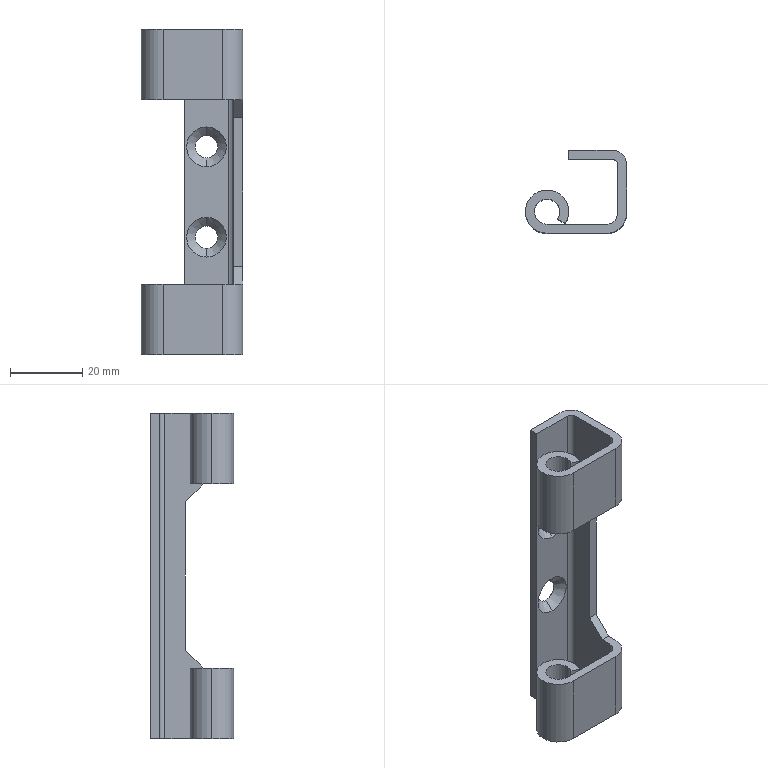Part | NX | features BREP 1 | 1 solid | 44 faces | box 28 x 23 x 90 mm | volume 10200 mm3 | cylinder 22 | plane 18 | cone 4 | commonest cylinder face diameters 7 x6 12 x6 6.2 x4 6 x2 11 x2 3 x1
STEP:
#1=CARTESIAN_POINT('',(6.,0.,-25.5));
#2=VERTEX_POINT('',#1);
#3=CARTESIAN_POINT('',(6.,0.,-45.));
#4=VERTEX_POINT('',#3);
#5=CARTESIAN_POINT('',(6.,0.,45.));
#6=DIRECTION('',(0.,0.,-1.));
#7=VECTOR('',#6,1000.);
#8=LINE('',#5,#7);
#9=EDGE_CURVE('',#2,#4,#8,.T.);
#10=ORIENTED_EDGE('',*,*,#9,.F.);
#11=CARTESIAN_POINT('',(5.029,-3.273,-25.5));
#12=VERTEX_POINT('',#11);
#13=CARTESIAN_POINT('',(0.0004653,0.,-25.5));
#14=DIRECTION('',(0.,0.,1.));
#15=DIRECTION('',(0.8381,-0.5456,0.));
#16=AXIS2_PLACEMENT_3D('',#13,#14,#15);
#17=CIRCLE('',#16,6.);
#18=EDGE_CURVE('',#12,#2,#17,.T.);
#19=ORIENTED_EDGE('',*,*,#18,.F.);
#20=CARTESIAN_POINT('',(5.029,-3.273,-45.));
#21=VERTEX_POINT('',#20);
#22=CARTESIAN_POINT('',(5.029,-3.273,-25.5));
#23=DIRECTION('',(0.,0.,-1.));
#24=VECTOR('',#23,1000.);
#25=LINE('',#22,#24);
#26=EDGE_CURVE('',#12,#21,#25,.T.);
#27=ORIENTED_EDGE('',*,*,#26,.T.);
#28=CARTESIAN_POINT('',(0.0004653,0.,-45.));
#29=DIRECTION('',(0.,0.,1.));
#30=DIRECTION('',(0.8381,-0.5456,0.));
#31=AXIS2_PLACEMENT_3D('',#28,#29,#30);
#32=CIRCLE('',#31,6.);
#33=EDGE_CURVE('',#21,#4,#32,.T.);
#34=ORIENTED_EDGE('',*,*,#33,.T.);
#35=EDGE_LOOP('',(#10,#19,#27,#34));
#36=FACE_BOUND('',#35,.T.);
#37=CARTESIAN_POINT('',(0.0004653,0.,45.));
#38=DIRECTION('',(0.,0.,-1.));
#39=DIRECTION('',(-1.,0.,0.));
#40=AXIS2_PLACEMENT_3D('',#37,#38,#39);
#41=CYLINDRICAL_SURFACE('',#40,6.);
#42=ADVANCED_FACE('',(#36),#41,.T.);
#43=CARTESIAN_POINT('',(16.5,-6.,-25.5));
#44=VERTEX_POINT('',#43);
#45=CARTESIAN_POINT('',(16.5,-6.,-45.));
#46=VERTEX_POINT('',#45);
#47=CARTESIAN_POINT('',(16.5,-6.,-25.5));
#48=DIRECTION('',(0.,0.,-1.));
#49=VECTOR('',#48,1000.);
#50=LINE('',#47,#49);
#51=EDGE_CURVE('',#44,#46,#50,.T.);
#52=ORIENTED_EDGE('',*,*,#51,.F.);
#53=CARTESIAN_POINT('',(0.0004653,-6.,-25.5));
#54=VERTEX_POINT('',#53);
#55=CARTESIAN_POINT('',(0.0004653,-6.,-25.5));
#56=DIRECTION('',(1.,0.,0.));
#57=VECTOR('',#56,1000.);
#58=LINE('',#55,#57);
#59=EDGE_CURVE('',#54,#44,#58,.T.);
#60=ORIENTED_EDGE('',*,*,#59,.F.);
#61=CARTESIAN_POINT('',(0.0004653,-6.,-45.));
#62=VERTEX_POINT('',#61);
#63=CARTESIAN_POINT('',(0.0004653,-6.,-25.5));
#64=DIRECTION('',(0.,0.,-1.));
#65=VECTOR('',#64,1000.);
#66=LINE('',#63,#65);
#67=EDGE_CURVE('',#54,#62,#66,.T.);
#68=ORIENTED_EDGE('',*,*,#67,.T.);
#69=CARTESIAN_POINT('',(0.0004653,-6.,-45.));
#70=DIRECTION('',(1.,0.,0.));
#71=VECTOR('',#70,1000.);
#72=LINE('',#69,#71);
#73=EDGE_CURVE('',#62,#46,#72,.T.);
#74=ORIENTED_EDGE('',*,*,#73,.T.);
#75=EDGE_LOOP('',(#52,#60,#68,#74));
#76=FACE_BOUND('',#75,.T.);
#77=CARTESIAN_POINT('',(0.0004653,-6.,45.));
#78=DIRECTION('',(0.,1.,0.));
#79=DIRECTION('',(0.,0.,1.));
#80=AXIS2_PLACEMENT_3D('',#77,#78,#79);
#81=PLANE('',#80);
#82=ADVANCED_FACE('',(#76),#81,.F.);
#83=CARTESIAN_POINT('',(16.5,-3.5,-25.5));
#84=VERTEX_POINT('',#83);
#85=CARTESIAN_POINT('',(0.0004653,-3.5,-25.5));
#86=VERTEX_POINT('',#85);
#87=CARTESIAN_POINT('',(16.5,-3.5,-25.5));
#88=DIRECTION('',(-1.,0.,0.));
#89=VECTOR('',#88,1000.);
#90=LINE('',#87,#89);
#91=EDGE_CURVE('',#84,#86,#90,.T.);
#92=ORIENTED_EDGE('',*,*,#91,.F.);
#93=CARTESIAN_POINT('',(16.5,-3.5,-45.));
#94=VERTEX_POINT('',#93);
#95=CARTESIAN_POINT('',(16.5,-3.5,-25.5));
#96=DIRECTION('',(0.,0.,-1.));
#97=VECTOR('',#96,1000.);
#98=LINE('',#95,#97);
#99=EDGE_CURVE('',#84,#94,#98,.T.);
#100=ORIENTED_EDGE('',*,*,#99,.T.);
#101=CARTESIAN_POINT('',(0.0004653,-3.5,-45.));
#102=VERTEX_POINT('',#101);
#103=CARTESIAN_POINT('',(16.5,-3.5,-45.));
#104=DIRECTION('',(-1.,0.,0.));
#105=VECTOR('',#104,1000.);
#106=LINE('',#103,#105);
#107=EDGE_CURVE('',#94,#102,#106,.T.);
#108=ORIENTED_EDGE('',*,*,#107,.T.);
#109=CARTESIAN_POINT('',(0.0004653,-3.5,-25.5));
#110=DIRECTION('',(0.,0.,-1.));
#111=VECTOR('',#110,1000.);
#112=LINE('',#109,#111);
#113=EDGE_CURVE('',#86,#102,#112,.T.);
#114=ORIENTED_EDGE('',*,*,#113,.F.);
#115=EDGE_LOOP('',(#92,#100,#108,#114));
#116=FACE_BOUND('',#115,.T.);
#117=CARTESIAN_POINT('',(16.5,-3.5,45.));
#118=DIRECTION('',(0.,-1.,0.));
#119=DIRECTION('',(0.,0.,-1.));
#120=AXIS2_PLACEMENT_3D('',#117,#118,#119);
#121=PLANE('',#120);
#122=ADVANCED_FACE('',(#116),#121,.F.);
#123=CARTESIAN_POINT('',(-3.5,0.000000072,-25.5));
#124=VERTEX_POINT('',#123);
#125=CARTESIAN_POINT('',(-3.5,0.000000072,-45.));
#126=VERTEX_POINT('',#125);
#127=CARTESIAN_POINT('',(-3.5,0.000000072,45.));
#128=DIRECTION('',(0.,0.,-1.));
#129=VECTOR('',#128,1000.);
#130=LINE('',#127,#129);
#131=EDGE_CURVE('',#124,#126,#130,.T.);
#132=ORIENTED_EDGE('',*,*,#131,.F.);
#133=CARTESIAN_POINT('',(0.0004654,0.000000072,-25.5));
#134=DIRECTION('',(0.,0.,1.));
#135=DIRECTION('',(0.8166,-0.5772,0.));
#136=AXIS2_PLACEMENT_3D('',#133,#134,#135);
#137=CIRCLE('',#136,3.5);
#138=EDGE_CURVE('',#124,#86,#137,.T.);
#139=ORIENTED_EDGE('',*,*,#138,.T.);
#140=ORIENTED_EDGE('',*,*,#113,.T.);
#141=CARTESIAN_POINT('',(0.0004654,0.000000072,-45.));
#142=DIRECTION('',(0.,0.,1.));
#143=DIRECTION('',(0.8166,-0.5772,0.));
#144=AXIS2_PLACEMENT_3D('',#141,#142,#143);
#145=CIRCLE('',#144,3.5);
#146=EDGE_CURVE('',#126,#102,#145,.T.);
#147=ORIENTED_EDGE('',*,*,#146,.F.);
#148=EDGE_LOOP('',(#132,#139,#140,#147));
#149=FACE_BOUND('',#148,.T.);
#150=CARTESIAN_POINT('',(0.0004654,0.000000072,45.));
#151=DIRECTION('',(0.,0.,-1.));
#152=DIRECTION('',(-1.,0.,0.));
#153=AXIS2_PLACEMENT_3D('',#150,#151,#152);
#154=CYLINDRICAL_SURFACE('',#153,3.5);
#155=ADVANCED_FACE('',(#149),#154,.F.);
#156=CARTESIAN_POINT('',(2.859,-2.02,-25.5));
#157=VERTEX_POINT('',#156);
#158=CARTESIAN_POINT('',(2.859,-2.02,-25.5));
#159=DIRECTION('',(0.866,-0.5,0.));
#160=VECTOR('',#159,1000.);
#161=LINE('',#158,#160);
#162=EDGE_CURVE('',#157,#12,#161,.T.);
#163=ORIENTED_EDGE('',*,*,#162,.F.);
#164=CARTESIAN_POINT('',(2.859,-2.02,-45.));
#165=VERTEX_POINT('',#164);
#166=CARTESIAN_POINT('',(2.859,-2.02,-25.5));
#167=DIRECTION('',(0.,0.,-1.));
#168=VECTOR('',#167,1000.);
#169=LINE('',#166,#168);
#170=EDGE_CURVE('',#157,#165,#169,.T.);
#171=ORIENTED_EDGE('',*,*,#170,.T.);
#172=CARTESIAN_POINT('',(2.859,-2.02,-45.));
#173=DIRECTION('',(0.866,-0.5,0.));
#174=VECTOR('',#173,1000.);
#175=LINE('',#172,#174);
#176=EDGE_CURVE('',#165,#21,#175,.T.);
#177=ORIENTED_EDGE('',*,*,#176,.T.);
#178=ORIENTED_EDGE('',*,*,#26,.F.);
#179=EDGE_LOOP('',(#163,#171,#177,#178));
#180=FACE_BOUND('',#179,.T.);
#181=CARTESIAN_POINT('',(2.859,-2.02,45.));
#182=DIRECTION('',(0.5,0.866,0.));
#183=DIRECTION('',(-0.866,0.5,0.));
#184=AXIS2_PLACEMENT_3D('',#181,#182,#183);
#185=PLANE('',#184);
#186=ADVANCED_FACE('',(#180),#185,.F.);
#187=CARTESIAN_POINT('',(12.,16.9,-9.4));
#188=VERTEX_POINT('',#187);
#189=CARTESIAN_POINT('',(12.,14.5,-7.));
#190=VERTEX_POINT('',#189);
#191=CARTESIAN_POINT('',(12.,16.9,-9.4));
#192=DIRECTION('',(0.,-0.7071,0.7071));
#193=VECTOR('',#192,1000.);
#194=LINE('',#191,#193);
#195=EDGE_CURVE('',#188,#190,#194,.T.);
#196=ORIENTED_EDGE('',*,*,#195,.F.);
#197=CARTESIAN_POINT('',(12.,16.9,-15.6));
#198=VERTEX_POINT('',#197);
#199=CARTESIAN_POINT('',(12.,16.9,-12.5));
#200=DIRECTION('',(0.,-1.,0.));
#201=DIRECTION('',(0.,0.,-1.));
#202=AXIS2_PLACEMENT_3D('',#199,#200,#201);
#203=CIRCLE('',#202,3.1);
#204=EDGE_CURVE('',#198,#188,#203,.T.);
#205=ORIENTED_EDGE('',*,*,#204,.F.);
#206=CARTESIAN_POINT('',(12.,14.5,-18.));
#207=VERTEX_POINT('',#206);
#208=CARTESIAN_POINT('',(12.,16.9,-15.6));
#209=DIRECTION('',(0.,-0.7071,-0.7071));
#210=VECTOR('',#209,1000.);
#211=LINE('',#208,#210);
#212=EDGE_CURVE('',#198,#207,#211,.T.);
#213=ORIENTED_EDGE('',*,*,#212,.T.);
#214=CARTESIAN_POINT('',(12.,14.5,-12.5));
#215=DIRECTION('',(0.,-1.,0.));
#216=DIRECTION('',(0.,0.,-1.));
#217=AXIS2_PLACEMENT_3D('',#214,#215,#216);
#218=CIRCLE('',#217,5.5);
#219=EDGE_CURVE('',#207,#190,#218,.T.);
#220=ORIENTED_EDGE('',*,*,#219,.T.);
#221=EDGE_LOOP('',(#196,#205,#213,#220));
#222=FACE_BOUND('',#221,.T.);
#223=CARTESIAN_POINT('',(12.,16.9,-12.5));
#224=DIRECTION('',(0.,-1.,0.));
#225=DIRECTION('',(0.,0.,-1.));
#226=AXIS2_PLACEMENT_3D('',#223,#224,#225);
#227=CONICAL_SURFACE('',#226,3.1,0.7854);
#228=ADVANCED_FACE('',(#222),#227,.F.);
#229=CARTESIAN_POINT('',(12.,16.9,15.6));
#230=VERTEX_POINT('',#229);
#231=CARTESIAN_POINT('',(12.,14.5,18.));
#232=VERTEX_POINT('',#231);
#233=CARTESIAN_POINT('',(12.,16.9,15.6));
#234=DIRECTION('',(0.,-0.7071,0.7071));
#235=VECTOR('',#234,1000.);
#236=LINE('',#233,#235);
#237=EDGE_CURVE('',#230,#232,#236,.T.);
#238=ORIENTED_EDGE('',*,*,#237,.F.);
#239=CARTESIAN_POINT('',(12.,16.9,9.4));
#240=VERTEX_POINT('',#239);
#241=CARTESIAN_POINT('',(12.,16.9,12.5));
#242=DIRECTION('',(0.,-1.,0.));
#243=DIRECTION('',(0.,0.,-1.));
#244=AXIS2_PLACEMENT_3D('',#241,#242,#243);
#245=CIRCLE('',#244,3.1);
#246=EDGE_CURVE('',#240,#230,#245,.T.);
#247=ORIENTED_EDGE('',*,*,#246,.F.);
#248=CARTESIAN_POINT('',(12.,14.5,7.));
#249=VERTEX_POINT('',#248);
#250=CARTESIAN_POINT('',(12.,16.9,9.4));
#251=DIRECTION('',(0.,-0.7071,-0.7071));
#252=VECTOR('',#251,1000.);
#253=LINE('',#250,#252);
#254=EDGE_CURVE('',#240,#249,#253,.T.);
#255=ORIENTED_EDGE('',*,*,#254,.T.);
#256=CARTESIAN_POINT('',(12.,14.5,12.5));
#257=DIRECTION('',(0.,-1.,0.));
#258=DIRECTION('',(0.,0.,-1.));
#259=AXIS2_PLACEMENT_3D('',#256,#257,#258);
#260=CIRCLE('',#259,5.5);
#261=EDGE_CURVE('',#249,#232,#260,.T.);
#262=ORIENTED_EDGE('',*,*,#261,.T.);
#263=EDGE_LOOP('',(#238,#247,#255,#262));
#264=FACE_BOUND('',#263,.T.);
#265=CARTESIAN_POINT('',(12.,16.9,12.5));
#266=DIRECTION('',(0.,-1.,0.));
#267=DIRECTION('',(0.,0.,-1.));
#268=AXIS2_PLACEMENT_3D('',#265,#266,#267);
#269=CONICAL_SURFACE('',#268,3.1,0.7854);
#270=ADVANCED_FACE('',(#264),#269,.F.);
#271=CARTESIAN_POINT('',(12.,17.,-9.4));
#272=VERTEX_POINT('',#271);
#273=CARTESIAN_POINT('',(12.,14.5,-9.4));
#274=DIRECTION('',(0.,-1.,0.));
#275=VECTOR('',#274,1000.);
#276=LINE('',#273,#275);
#277=EDGE_CURVE('',#272,#188,#276,.T.);
#278=ORIENTED_EDGE('',*,*,#277,.F.);
#279=CARTESIAN_POINT('',(12.,17.,-15.6));
#280=VERTEX_POINT('',#279);
#281=CARTESIAN_POINT('',(12.,17.,-12.5));
#282=DIRECTION('',(0.,1.,0.));
#283=DIRECTION('',(0.,0.,-1.));
#284=AXIS2_PLACEMENT_3D('',#281,#282,#283);
#285=CIRCLE('',#284,3.1);
#286=EDGE_CURVE('',#272,#280,#285,.T.);
#287=ORIENTED_EDGE('',*,*,#286,.T.);
#288=CARTESIAN_POINT('',(12.,14.5,-15.6));
#289=DIRECTION('',(0.,-1.,0.));
#290=VECTOR('',#289,1000.);
#291=LINE('',#288,#290);
#292=EDGE_CURVE('',#280,#198,#291,.T.);
#293=ORIENTED_EDGE('',*,*,#292,.T.);
#294=ORIENTED_EDGE('',*,*,#204,.T.);
#295=EDGE_LOOP('',(#278,#287,#293,#294));
#296=FACE_BOUND('',#295,.T.);
#297=CARTESIAN_POINT('',(12.,14.5,-12.5));
#298=DIRECTION('',(0.,-1.,0.));
#299=DIRECTION('',(0.,0.,-1.));
#300=AXIS2_PLACEMENT_3D('',#297,#298,#299);
#301=CYLINDRICAL_SURFACE('',#300,3.1);
#302=ADVANCED_FACE('',(#296),#301,.F.);
#303=CARTESIAN_POINT('',(12.,17.,15.6));
#304=VERTEX_POINT('',#303);
#305=CARTESIAN_POINT('',(12.,14.5,15.6));
#306=DIRECTION('',(0.,-1.,0.));
#307=VECTOR('',#306,1000.);
#308=LINE('',#305,#307);
#309=EDGE_CURVE('',#304,#230,#308,.T.);
#310=ORIENTED_EDGE('',*,*,#309,.F.);
#311=CARTESIAN_POINT('',(12.,17.,9.4));
#312=VERTEX_POINT('',#311);
#313=CARTESIAN_POINT('',(12.,17.,12.5));
#314=DIRECTION('',(0.,1.,0.));
#315=DIRECTION('',(0.,0.,-1.));
#316=AXIS2_PLACEMENT_3D('',#313,#314,#315);
#317=CIRCLE('',#316,3.1);
#318=EDGE_CURVE('',#304,#312,#317,.T.);
#319=ORIENTED_EDGE('',*,*,#318,.T.);
#320=CARTESIAN_POINT('',(12.,14.5,9.4));
#321=DIRECTION('',(0.,-1.,0.));
#322=VECTOR('',#321,1000.);
#323=LINE('',#320,#322);
#324=EDGE_CURVE('',#312,#240,#323,.T.);
#325=ORIENTED_EDGE('',*,*,#324,.T.);
#326=ORIENTED_EDGE('',*,*,#246,.T.);
#327=EDGE_LOOP('',(#310,#319,#325,#326));
#328=FACE_BOUND('',#327,.T.);
#329=CARTESIAN_POINT('',(12.,14.5,12.5));
#330=DIRECTION('',(0.,-1.,0.));
#331=DIRECTION('',(0.,0.,-1.));
#332=AXIS2_PLACEMENT_3D('',#329,#330,#331);
#333=CYLINDRICAL_SURFACE('',#332,3.1);
#334=ADVANCED_FACE('',(#328),#333,.F.);
#335=CARTESIAN_POINT('',(22.,-0.5,-25.5));
#336=VERTEX_POINT('',#335);
#337=CARTESIAN_POINT('',(16.5,-0.5,-25.5));
#338=DIRECTION('',(0.,0.,1.));
#339=DIRECTION('',(0.,-1.,0.));
#340=AXIS2_PLACEMENT_3D('',#337,#338,#339);
#341=CIRCLE('',#340,5.5);
#342=EDGE_CURVE('',#44,#336,#341,.T.);
#343=ORIENTED_EDGE('',*,*,#342,.F.);
#344=ORIENTED_EDGE('',*,*,#51,.T.);
#345=CARTESIAN_POINT('',(22.,-0.5,-45.));
#346=VERTEX_POINT('',#345);
#347=CARTESIAN_POINT('',(16.5,-0.5,-45.));
#348=DIRECTION('',(0.,0.,1.));
#349=DIRECTION('',(0.,-1.,0.));
#350=AXIS2_PLACEMENT_3D('',#347,#348,#349);
#351=CIRCLE('',#350,5.5);
#352=EDGE_CURVE('',#46,#346,#351,.T.);
#353=ORIENTED_EDGE('',*,*,#352,.T.);
#354=CARTESIAN_POINT('',(22.,-0.5,-25.5));
#355=DIRECTION('',(0.,0.,-1.));
#356=VECTOR('',#355,1000.);
#357=LINE('',#354,#356);
#358=EDGE_CURVE('',#336,#346,#357,.T.);
#359=ORIENTED_EDGE('',*,*,#358,.F.);
#360=EDGE_LOOP('',(#343,#344,#353,#359));
#361=FACE_BOUND('',#360,.T.);
#362=CARTESIAN_POINT('',(16.5,-0.5,45.));
#363=DIRECTION('',(0.,0.,-1.));
#364=DIRECTION('',(-1.,0.,0.));
#365=AXIS2_PLACEMENT_3D('',#362,#363,#364);
#366=CYLINDRICAL_SURFACE('',#365,5.5);
#367=ADVANCED_FACE('',(#361),#366,.T.);
#368=CARTESIAN_POINT('',(22.,7.3,-20.55));
#369=VERTEX_POINT('',#368);
#370=CARTESIAN_POINT('',(22.,7.3,20.55));
#371=VERTEX_POINT('',#370);
#372=CARTESIAN_POINT('',(22.,7.3,-20.55));
#373=DIRECTION('',(0.,0.,1.));
#374=VECTOR('',#373,1000.);
#375=LINE('',#372,#374);
#376=EDGE_CURVE('',#369,#371,#375,.T.);
#377=ORIENTED_EDGE('',*,*,#376,.T.);
#378=CARTESIAN_POINT('',(19.5,7.3,20.55));
#379=VERTEX_POINT('',#378);
#380=CARTESIAN_POINT('',(22.,7.3,20.55));
#381=DIRECTION('',(-1.,0.,0.));
#382=VECTOR('',#381,1000.);
#383=LINE('',#380,#382);
#384=EDGE_CURVE('',#371,#379,#383,.T.);
#385=ORIENTED_EDGE('',*,*,#384,.T.);
#386=CARTESIAN_POINT('',(19.5,7.3,-20.55));
#387=VERTEX_POINT('',#386);
#388=CARTESIAN_POINT('',(19.5,7.3,20.55));
#389=DIRECTION('',(0.,0.,-1.));
#390=VECTOR('',#389,1000.);
#391=LINE('',#388,#390);
#392=EDGE_CURVE('',#379,#387,#391,.T.);
#393=ORIENTED_EDGE('',*,*,#392,.T.);
#394=CARTESIAN_POINT('',(22.,7.3,-20.55));
#395=DIRECTION('',(-1.,0.,0.));
#396=VECTOR('',#395,1000.);
#397=LINE('',#394,#396);
#398=EDGE_CURVE('',#369,#387,#397,.T.);
#399=ORIENTED_EDGE('',*,*,#398,.F.);
#400=EDGE_LOOP('',(#377,#385,#393,#399));
#401=FACE_BOUND('',#400,.T.);
#402=CARTESIAN_POINT('',(60.,7.3,-20.55));
#403=DIRECTION('',(0.,-1.,0.));
#404=DIRECTION('',(0.,0.,-1.));
#405=AXIS2_PLACEMENT_3D('',#402,#403,#404);
#406=PLANE('',#405);
#407=ADVANCED_FACE('',(#401),#406,.T.);
#408=CARTESIAN_POINT('',(22.,2.35,-25.5));
#409=VERTEX_POINT('',#408);
#410=CARTESIAN_POINT('',(22.,2.35,-25.5));
#411=DIRECTION('',(0.,0.7071,0.7071));
#412=VECTOR('',#411,1000.);
#413=LINE('',#410,#412);
#414=EDGE_CURVE('',#409,#369,#413,.T.);
#415=ORIENTED_EDGE('',*,*,#414,.T.);
#416=ORIENTED_EDGE('',*,*,#398,.T.);
#417=CARTESIAN_POINT('',(19.5,2.35,-25.5));
#418=VERTEX_POINT('',#417);
#419=CARTESIAN_POINT('',(19.5,7.3,-20.55));
#420=DIRECTION('',(0.,-0.7071,-0.7071));
#421=VECTOR('',#420,1000.);
#422=LINE('',#419,#421);
#423=EDGE_CURVE('',#387,#418,#422,.T.);
#424=ORIENTED_EDGE('',*,*,#423,.T.);
#425=CARTESIAN_POINT('',(22.,2.35,-25.5));
#426=DIRECTION('',(-1.,0.,0.));
#427=VECTOR('',#426,1000.);
#428=LINE('',#425,#427);
#429=EDGE_CURVE('',#409,#418,#428,.T.);
#430=ORIENTED_EDGE('',*,*,#429,.F.);
#431=EDGE_LOOP('',(#415,#416,#424,#430));
#432=FACE_BOUND('',#431,.T.);
#433=CARTESIAN_POINT('',(60.,2.35,-25.5));
#434=DIRECTION('',(0.,-0.7071,0.7071));
#435=DIRECTION('',(0.,-0.7071,-0.7071));
#436=AXIS2_PLACEMENT_3D('',#433,#434,#435);
#437=PLANE('',#436);
#438=ADVANCED_FACE('',(#432),#437,.T.);
#439=ORIENTED_EDGE('',*,*,#59,.T.);
#440=ORIENTED_EDGE('',*,*,#342,.T.);
#441=CARTESIAN_POINT('',(22.,-0.5,-25.5));
#442=DIRECTION('',(0.,1.,0.));
#443=VECTOR('',#442,1000.);
#444=LINE('',#441,#443);
#445=EDGE_CURVE('',#336,#409,#444,.T.);
#446=ORIENTED_EDGE('',*,*,#445,.T.);
#447=ORIENTED_EDGE('',*,*,#429,.T.);
#448=CARTESIAN_POINT('',(19.5,-0.5,-25.5));
#449=VERTEX_POINT('',#448);
#450=CARTESIAN_POINT('',(19.5,2.35,-25.5));
#451=DIRECTION('',(0.,-1.,0.));
#452=VECTOR('',#451,1000.);
#453=LINE('',#450,#452);
#454=EDGE_CURVE('',#418,#449,#453,.T.);
#455=ORIENTED_EDGE('',*,*,#454,.T.);
#456=CARTESIAN_POINT('',(16.5,-0.5,-25.5));
#457=DIRECTION('',(0.,0.,1.));
#458=DIRECTION('',(0.,-1.,0.));
#459=AXIS2_PLACEMENT_3D('',#456,#457,#458);
#460=CIRCLE('',#459,3.);
#461=EDGE_CURVE('',#84,#449,#460,.T.);
#462=ORIENTED_EDGE('',*,*,#461,.F.);
#463=ORIENTED_EDGE('',*,*,#91,.T.);
#464=ORIENTED_EDGE('',*,*,#138,.F.);
#465=CARTESIAN_POINT('',(3.5,0.000000072,-25.5));
#466=VERTEX_POINT('',#465);
#467=CARTESIAN_POINT('',(0.0004654,0.000000072,-25.5));
#468=DIRECTION('',(0.,0.,1.));
#469=DIRECTION('',(0.8166,-0.5772,0.));
#470=AXIS2_PLACEMENT_3D('',#467,#468,#469);
#471=CIRCLE('',#470,3.5);
#472=EDGE_CURVE('',#466,#124,#471,.T.);
#473=ORIENTED_EDGE('',*,*,#472,.F.);
#474=CARTESIAN_POINT('',(0.0004654,0.000000072,-25.5));
#475=DIRECTION('',(0.,0.,1.));
#476=DIRECTION('',(0.8166,-0.5772,0.));
#477=AXIS2_PLACEMENT_3D('',#474,#475,#476);
#478=CIRCLE('',#477,3.5);
#479=EDGE_CURVE('',#157,#466,#478,.T.);
#480=ORIENTED_EDGE('',*,*,#479,.F.);
#481=ORIENTED_EDGE('',*,*,#162,.T.);
#482=ORIENTED_EDGE('',*,*,#18,.T.);
#483=CARTESIAN_POINT('',(-6.,0.,-25.5));
#484=VERTEX_POINT('',#483);
#485=CARTESIAN_POINT('',(0.0004653,0.,-25.5));
#486=DIRECTION('',(0.,0.,1.));
#487=DIRECTION('',(0.8381,-0.5456,0.));
#488=AXIS2_PLACEMENT_3D('',#485,#486,#487);
#489=CIRCLE('',#488,6.);
#490=EDGE_CURVE('',#2,#484,#489,.T.);
#491=ORIENTED_EDGE('',*,*,#490,.T.);
#492=CARTESIAN_POINT('',(0.0004653,0.,-25.5));
#493=DIRECTION('',(0.,0.,1.));
#494=DIRECTION('',(0.8381,-0.5456,0.));
#495=AXIS2_PLACEMENT_3D('',#492,#493,#494);
#496=CIRCLE('',#495,6.);
#497=EDGE_CURVE('',#484,#54,#496,.T.);
#498=ORIENTED_EDGE('',*,*,#497,.T.);
#499=EDGE_LOOP('',(#439,#440,#446,#447,#455,#462,#463,#464,#473,#480,#481,#482,#491,#498));
#500=FACE_BOUND('',#499,.T.);
#501=CARTESIAN_POINT('',(10.,-6.55,-25.5));
#502=DIRECTION('',(0.,0.,1.));
#503=DIRECTION('',(1.,0.,0.));
#504=AXIS2_PLACEMENT_3D('',#501,#502,#503);
#505=PLANE('',#504);
#506=ADVANCED_FACE('',(#500),#505,.T.);
#507=ORIENTED_EDGE('',*,*,#99,.F.);
#508=ORIENTED_EDGE('',*,*,#461,.T.);
#509=CARTESIAN_POINT('',(19.5,-0.5,-45.));
#510=VERTEX_POINT('',#509);
#511=CARTESIAN_POINT('',(19.5,-0.5,-25.5));
#512=DIRECTION('',(0.,0.,-1.));
#513=VECTOR('',#512,1000.);
#514=LINE('',#511,#513);
#515=EDGE_CURVE('',#449,#510,#514,.T.);
#516=ORIENTED_EDGE('',*,*,#515,.T.);
#517=CARTESIAN_POINT('',(16.5,-0.5,-45.));
#518=DIRECTION('',(0.,0.,1.));
#519=DIRECTION('',(0.,-1.,0.));
#520=AXIS2_PLACEMENT_3D('',#517,#518,#519);
#521=CIRCLE('',#520,3.);
#522=EDGE_CURVE('',#94,#510,#521,.T.);
#523=ORIENTED_EDGE('',*,*,#522,.F.);
#524=EDGE_LOOP('',(#507,#508,#516,#523));
#525=FACE_BOUND('',#524,.T.);
#526=CARTESIAN_POINT('',(16.5,-0.5,45.));
#527=DIRECTION('',(0.,0.,-1.));
#528=DIRECTION('',(-1.,0.,0.));
#529=AXIS2_PLACEMENT_3D('',#526,#527,#528);
#530=CYLINDRICAL_SURFACE('',#529,3.);
#531=ADVANCED_FACE('',(#525),#530,.F.);
#532=ORIENTED_EDGE('',*,*,#176,.F.);
#533=CARTESIAN_POINT('',(3.5,0.000000072,-45.));
#534=VERTEX_POINT('',#533);
#535=CARTESIAN_POINT('',(0.0004654,0.000000072,-45.));
#536=DIRECTION('',(0.,0.,1.));
#537=DIRECTION('',(0.8166,-0.5772,0.));
#538=AXIS2_PLACEMENT_3D('',#535,#536,#537);
#539=CIRCLE('',#538,3.5);
#540=EDGE_CURVE('',#165,#534,#539,.T.);
#541=ORIENTED_EDGE('',*,*,#540,.T.);
#542=CARTESIAN_POINT('',(0.0004654,0.000000072,-45.));
#543=DIRECTION('',(0.,0.,1.));
#544=DIRECTION('',(0.8166,-0.5772,0.));
#545=AXIS2_PLACEMENT_3D('',#542,#543,#544);
#546=CIRCLE('',#545,3.5);
#547=EDGE_CURVE('',#534,#126,#546,.T.);
#548=ORIENTED_EDGE('',*,*,#547,.T.);
#549=ORIENTED_EDGE('',*,*,#146,.T.);
#550=ORIENTED_EDGE('',*,*,#107,.F.);
#551=ORIENTED_EDGE('',*,*,#522,.T.);
#552=CARTESIAN_POINT('',(19.5,13.,-45.));
#553=VERTEX_POINT('',#552);
#554=CARTESIAN_POINT('',(19.5,13.,-45.));
#555=DIRECTION('',(0.,-1.,0.));
#556=VECTOR('',#555,1000.);
#557=LINE('',#554,#556);
#558=EDGE_CURVE('',#553,#510,#557,.T.);
#559=ORIENTED_EDGE('',*,*,#558,.F.);
#560=CARTESIAN_POINT('',(18.,14.5,-45.));
#561=VERTEX_POINT('',#560);
#562=CARTESIAN_POINT('',(18.,13.,-45.));
#563=DIRECTION('',(0.,0.,1.));
#564=DIRECTION('',(1.,0.,0.));
#565=AXIS2_PLACEMENT_3D('',#562,#563,#564);
#566=CIRCLE('',#565,1.5);
#567=EDGE_CURVE('',#553,#561,#566,.T.);
#568=ORIENTED_EDGE('',*,*,#567,.T.);
#569=CARTESIAN_POINT('',(6.,14.5,-45.));
#570=VERTEX_POINT('',#569);
#571=CARTESIAN_POINT('',(6.,14.5,-45.));
#572=DIRECTION('',(1.,0.,0.));
#573=VECTOR('',#572,1000.);
#574=LINE('',#571,#573);
#575=EDGE_CURVE('',#570,#561,#574,.T.);
#576=ORIENTED_EDGE('',*,*,#575,.F.);
#577=CARTESIAN_POINT('',(6.,17.,-45.));
#578=VERTEX_POINT('',#577);
#579=CARTESIAN_POINT('',(6.,17.,-45.));
#580=DIRECTION('',(0.,-1.,0.));
#581=VECTOR('',#580,1000.);
#582=LINE('',#579,#581);
#583=EDGE_CURVE('',#578,#570,#582,.T.);
#584=ORIENTED_EDGE('',*,*,#583,.F.);
#585=CARTESIAN_POINT('',(18.,17.,-45.));
#586=VERTEX_POINT('',#585);
#587=CARTESIAN_POINT('',(18.,17.,-45.));
#588=DIRECTION('',(-1.,0.,0.));
#589=VECTOR('',#588,1000.);
#590=LINE('',#587,#589);
#591=EDGE_CURVE('',#586,#578,#590,.T.);
#592=ORIENTED_EDGE('',*,*,#591,.F.);
#593=CARTESIAN_POINT('',(22.,13.,-45.));
#594=VERTEX_POINT('',#593);
#595=CARTESIAN_POINT('',(18.,13.,-45.));
#596=DIRECTION('',(0.,0.,1.));
#597=DIRECTION('',(1.,0.,0.));
#598=AXIS2_PLACEMENT_3D('',#595,#596,#597);
#599=CIRCLE('',#598,4.);
#600=EDGE_CURVE('',#594,#586,#599,.T.);
#601=ORIENTED_EDGE('',*,*,#600,.F.);
#602=CARTESIAN_POINT('',(22.,-0.5,-45.));
#603=DIRECTION('',(0.,1.,0.));
#604=VECTOR('',#603,1000.);
#605=LINE('',#602,#604);
#606=EDGE_CURVE('',#346,#594,#605,.T.);
#607=ORIENTED_EDGE('',*,*,#606,.F.);
#608=ORIENTED_EDGE('',*,*,#352,.F.);
#609=ORIENTED_EDGE('',*,*,#73,.F.);
#610=CARTESIAN_POINT('',(-6.,0.,-45.));
#611=VERTEX_POINT('',#610);
#612=CARTESIAN_POINT('',(0.0004653,0.,-45.));
#613=DIRECTION('',(0.,0.,1.));
#614=DIRECTION('',(0.8381,-0.5456,0.));
#615=AXIS2_PLACEMENT_3D('',#612,#613,#614);
#616=CIRCLE('',#615,6.);
#617=EDGE_CURVE('',#611,#62,#616,.T.);
#618=ORIENTED_EDGE('',*,*,#617,.F.);
#619=CARTESIAN_POINT('',(0.0004653,0.,-45.));
#620=DIRECTION('',(0.,0.,1.));
#621=DIRECTION('',(0.8381,-0.5456,0.));
#622=AXIS2_PLACEMENT_3D('',#619,#620,#621);
#623=CIRCLE('',#622,6.);
#624=EDGE_CURVE('',#4,#611,#623,.T.);
#625=ORIENTED_EDGE('',*,*,#624,.F.);
#626=ORIENTED_EDGE('',*,*,#33,.F.);
#627=EDGE_LOOP('',(#532,#541,#548,#549,#550,#551,#559,#568,#576,#584,#592,#601,#607,#608,#609,#618,#625,#626));
#628=FACE_BOUND('',#627,.T.);
#629=CARTESIAN_POINT('',(0.0004653,0.,-45.));
#630=DIRECTION('',(0.,0.,1.));
#631=DIRECTION('',(1.,0.,0.));
#632=AXIS2_PLACEMENT_3D('',#629,#630,#631);
#633=PLANE('',#632);
#634=ADVANCED_FACE('',(#628),#633,.F.);
#635=ORIENTED_EDGE('',*,*,#567,.F.);
#636=CARTESIAN_POINT('',(19.5,13.,45.));
#637=VERTEX_POINT('',#636);
#638=CARTESIAN_POINT('',(19.5,13.,45.));
#639=DIRECTION('',(0.,0.,-1.));
#640=VECTOR('',#639,1000.);
#641=LINE('',#638,#640);
#642=EDGE_CURVE('',#637,#553,#641,.T.);
#643=ORIENTED_EDGE('',*,*,#642,.F.);
#644=CARTESIAN_POINT('',(18.,14.5,45.));
#645=VERTEX_POINT('',#644);
#646=CARTESIAN_POINT('',(18.,13.,45.));
#647=DIRECTION('',(0.,0.,1.));
#648=DIRECTION('',(1.,0.,0.));
#649=AXIS2_PLACEMENT_3D('',#646,#647,#648);
#650=CIRCLE('',#649,1.5);
#651=EDGE_CURVE('',#637,#645,#650,.T.);
#652=ORIENTED_EDGE('',*,*,#651,.T.);
#653=CARTESIAN_POINT('',(18.,14.5,45.));
#654=DIRECTION('',(0.,0.,-1.));
#655=VECTOR('',#654,1000.);
#656=LINE('',#653,#655);
#657=EDGE_CURVE('',#645,#561,#656,.T.);
#658=ORIENTED_EDGE('',*,*,#657,.T.);
#659=EDGE_LOOP('',(#635,#643,#652,#658));
#660=FACE_BOUND('',#659,.T.);
#661=CARTESIAN_POINT('',(18.,13.,45.));
#662=DIRECTION('',(0.,0.,-1.));
#663=DIRECTION('',(-1.,0.,0.));
#664=AXIS2_PLACEMENT_3D('',#661,#662,#663);
#665=CYLINDRICAL_SURFACE('',#664,1.5);
#666=ADVANCED_FACE('',(#660),#665,.F.);
#667=ORIENTED_EDGE('',*,*,#575,.T.);
#668=ORIENTED_EDGE('',*,*,#657,.F.);
#669=CARTESIAN_POINT('',(6.,14.5,45.));
#670=VERTEX_POINT('',#669);
#671=CARTESIAN_POINT('',(6.,14.5,45.));
#672=DIRECTION('',(1.,0.,0.));
#673=VECTOR('',#672,1000.);
#674=LINE('',#671,#673);
#675=EDGE_CURVE('',#670,#645,#674,.T.);
#676=ORIENTED_EDGE('',*,*,#675,.F.);
#677=CARTESIAN_POINT('',(6.,14.5,45.));
#678=DIRECTION('',(0.,0.,-1.));
#679=VECTOR('',#678,1000.);
#680=LINE('',#677,#679);
#681=EDGE_CURVE('',#670,#570,#680,.T.);
#682=ORIENTED_EDGE('',*,*,#681,.T.);
#683=EDGE_LOOP('',(#667,#668,#676,#682));
#684=FACE_BOUND('',#683,.T.);
#685=ORIENTED_EDGE('',*,*,#219,.F.);
#686=CARTESIAN_POINT('',(12.,14.5,-12.5));
#687=DIRECTION('',(0.,-1.,0.));
#688=DIRECTION('',(0.,0.,-1.));
#689=AXIS2_PLACEMENT_3D('',#686,#687,#688);
#690=CIRCLE('',#689,5.5);
#691=EDGE_CURVE('',#190,#207,#690,.T.);
#692=ORIENTED_EDGE('',*,*,#691,.F.);
#693=EDGE_LOOP('',(#685,#692));
#694=FACE_BOUND('',#693,.T.);
#695=ORIENTED_EDGE('',*,*,#261,.F.);
#696=CARTESIAN_POINT('',(12.,14.5,12.5));
#697=DIRECTION('',(0.,-1.,0.));
#698=DIRECTION('',(0.,0.,-1.));
#699=AXIS2_PLACEMENT_3D('',#696,#697,#698);
#700=CIRCLE('',#699,5.5);
#701=EDGE_CURVE('',#232,#249,#700,.T.);
#702=ORIENTED_EDGE('',*,*,#701,.F.);
#703=EDGE_LOOP('',(#695,#702));
#704=FACE_BOUND('',#703,.T.);
#705=CARTESIAN_POINT('',(6.,14.5,45.));
#706=DIRECTION('',(0.,1.,0.));
#707=DIRECTION('',(0.,0.,1.));
#708=AXIS2_PLACEMENT_3D('',#705,#706,#707);
#709=PLANE('',#708);
#710=ADVANCED_FACE('',(#684,#694,#704),#709,.F.);
#711=ORIENTED_EDGE('',*,*,#583,.T.);
#712=ORIENTED_EDGE('',*,*,#681,.F.);
#713=CARTESIAN_POINT('',(6.,17.,45.));
#714=VERTEX_POINT('',#713);
#715=CARTESIAN_POINT('',(6.,17.,45.));
#716=DIRECTION('',(0.,-1.,0.));
#717=VECTOR('',#716,1000.);
#718=LINE('',#715,#717);
#719=EDGE_CURVE('',#714,#670,#718,.T.);
#720=ORIENTED_EDGE('',*,*,#719,.F.);
#721=CARTESIAN_POINT('',(6.,17.,45.));
#722=DIRECTION('',(0.,0.,-1.));
#723=VECTOR('',#722,1000.);
#724=LINE('',#721,#723);
#725=EDGE_CURVE('',#714,#578,#724,.T.);
#726=ORIENTED_EDGE('',*,*,#725,.T.);
#727=EDGE_LOOP('',(#711,#712,#720,#726));
#728=FACE_BOUND('',#727,.T.);
#729=CARTESIAN_POINT('',(6.,17.,45.));
#730=DIRECTION('',(1.,0.,0.));
#731=DIRECTION('',(0.,0.,-1.));
#732=AXIS2_PLACEMENT_3D('',#729,#730,#731);
#733=PLANE('',#732);
#734=ADVANCED_FACE('',(#728),#733,.F.);
#735=ORIENTED_EDGE('',*,*,#591,.T.);
#736=ORIENTED_EDGE('',*,*,#725,.F.);
#737=CARTESIAN_POINT('',(18.,17.,45.));
#738=VERTEX_POINT('',#737);
#739=CARTESIAN_POINT('',(18.,17.,45.));
#740=DIRECTION('',(-1.,0.,0.));
#741=VECTOR('',#740,1000.);
#742=LINE('',#739,#741);
#743=EDGE_CURVE('',#738,#714,#742,.T.);
#744=ORIENTED_EDGE('',*,*,#743,.F.);
#745=CARTESIAN_POINT('',(18.,17.,45.));
#746=DIRECTION('',(0.,0.,-1.));
#747=VECTOR('',#746,1000.);
#748=LINE('',#745,#747);
#749=EDGE_CURVE('',#738,#586,#748,.T.);
#750=ORIENTED_EDGE('',*,*,#749,.T.);
#751=EDGE_LOOP('',(#735,#736,#744,#750));
#752=FACE_BOUND('',#751,.T.);
#753=CARTESIAN_POINT('',(12.,17.,-12.5));
#754=DIRECTION('',(0.,1.,0.));
#755=DIRECTION('',(0.,0.,-1.));
#756=AXIS2_PLACEMENT_3D('',#753,#754,#755);
#757=CIRCLE('',#756,3.1);
#758=EDGE_CURVE('',#280,#272,#757,.T.);
#759=ORIENTED_EDGE('',*,*,#758,.F.);
#760=ORIENTED_EDGE('',*,*,#286,.F.);
#761=EDGE_LOOP('',(#759,#760));
#762=FACE_BOUND('',#761,.T.);
#763=CARTESIAN_POINT('',(12.,17.,12.5));
#764=DIRECTION('',(0.,1.,0.));
#765=DIRECTION('',(0.,0.,-1.));
#766=AXIS2_PLACEMENT_3D('',#763,#764,#765);
#767=CIRCLE('',#766,3.1);
#768=EDGE_CURVE('',#312,#304,#767,.T.);
#769=ORIENTED_EDGE('',*,*,#768,.F.);
#770=ORIENTED_EDGE('',*,*,#318,.F.);
#771=EDGE_LOOP('',(#769,#770));
#772=FACE_BOUND('',#771,.T.);
#773=CARTESIAN_POINT('',(18.,17.,45.));
#774=DIRECTION('',(0.,-1.,0.));
#775=DIRECTION('',(0.,0.,-1.));
#776=AXIS2_PLACEMENT_3D('',#773,#774,#775);
#777=PLANE('',#776);
#778=ADVANCED_FACE('',(#752,#762,#772),#777,.F.);
#779=ORIENTED_EDGE('',*,*,#600,.T.);
#780=ORIENTED_EDGE('',*,*,#749,.F.);
#781=CARTESIAN_POINT('',(22.,13.,45.));
#782=VERTEX_POINT('',#781);
#783=CARTESIAN_POINT('',(18.,13.,45.));
#784=DIRECTION('',(0.,0.,1.));
#785=DIRECTION('',(1.,0.,0.));
#786=AXIS2_PLACEMENT_3D('',#783,#784,#785);
#787=CIRCLE('',#786,4.);
#788=EDGE_CURVE('',#782,#738,#787,.T.);
#789=ORIENTED_EDGE('',*,*,#788,.F.);
#790=CARTESIAN_POINT('',(22.,13.,45.));
#791=DIRECTION('',(0.,0.,-1.));
#792=VECTOR('',#791,1000.);
#793=LINE('',#790,#792);
#794=EDGE_CURVE('',#782,#594,#793,.T.);
#795=ORIENTED_EDGE('',*,*,#794,.T.);
#796=EDGE_LOOP('',(#779,#780,#789,#795));
#797=FACE_BOUND('',#796,.T.);
#798=CARTESIAN_POINT('',(18.,13.,45.));
#799=DIRECTION('',(0.,0.,-1.));
#800=DIRECTION('',(-1.,0.,0.));
#801=AXIS2_PLACEMENT_3D('',#798,#799,#800);
#802=CYLINDRICAL_SURFACE('',#801,4.);
#803=ADVANCED_FACE('',(#797),#802,.T.);
#804=CARTESIAN_POINT('',(22.,2.35,25.5));
#805=VERTEX_POINT('',#804);
#806=CARTESIAN_POINT('',(22.,-0.5,25.5));
#807=VERTEX_POINT('',#806);
#808=CARTESIAN_POINT('',(22.,2.35,25.5));
#809=DIRECTION('',(0.,-1.,0.));
#810=VECTOR('',#809,1000.);
#811=LINE('',#808,#810);
#812=EDGE_CURVE('',#805,#807,#811,.T.);
#813=ORIENTED_EDGE('',*,*,#812,.F.);
#814=CARTESIAN_POINT('',(22.,7.3,20.55));
#815=DIRECTION('',(0.,-0.7071,0.7071));
#816=VECTOR('',#815,1000.);
#817=LINE('',#814,#816);
#818=EDGE_CURVE('',#371,#805,#817,.T.);
#819=ORIENTED_EDGE('',*,*,#818,.F.);
#820=ORIENTED_EDGE('',*,*,#376,.F.);
#821=ORIENTED_EDGE('',*,*,#414,.F.);
#822=ORIENTED_EDGE('',*,*,#445,.F.);
#823=ORIENTED_EDGE('',*,*,#358,.T.);
#824=ORIENTED_EDGE('',*,*,#606,.T.);
#825=ORIENTED_EDGE('',*,*,#794,.F.);
#826=CARTESIAN_POINT('',(22.,-0.5,45.));
#827=VERTEX_POINT('',#826);
#828=CARTESIAN_POINT('',(22.,-0.5,45.));
#829=DIRECTION('',(0.,1.,0.));
#830=VECTOR('',#829,1000.);
#831=LINE('',#828,#830);
#832=EDGE_CURVE('',#827,#782,#831,.T.);
#833=ORIENTED_EDGE('',*,*,#832,.F.);
#834=CARTESIAN_POINT('',(22.,-0.5,45.));
#835=DIRECTION('',(0.,0.,-1.));
#836=VECTOR('',#835,1000.);
#837=LINE('',#834,#836);
#838=EDGE_CURVE('',#827,#807,#837,.T.);
#839=ORIENTED_EDGE('',*,*,#838,.T.);
#840=EDGE_LOOP('',(#813,#819,#820,#821,#822,#823,#824,#825,#833,#839));
#841=FACE_BOUND('',#840,.T.);
#842=CARTESIAN_POINT('',(22.,-0.5,45.));
#843=DIRECTION('',(-1.,0.,0.));
#844=DIRECTION('',(0.,0.,1.));
#845=AXIS2_PLACEMENT_3D('',#842,#843,#844);
#846=PLANE('',#845);
#847=ADVANCED_FACE('',(#841),#846,.F.);
#848=ORIENTED_EDGE('',*,*,#818,.T.);
#849=CARTESIAN_POINT('',(19.5,2.35,25.5));
#850=VERTEX_POINT('',#849);
#851=CARTESIAN_POINT('',(22.,2.35,25.5));
#852=DIRECTION('',(-1.,0.,0.));
#853=VECTOR('',#852,1000.);
#854=LINE('',#851,#853);
#855=EDGE_CURVE('',#805,#850,#854,.T.);
#856=ORIENTED_EDGE('',*,*,#855,.T.);
#857=CARTESIAN_POINT('',(19.5,2.35,25.5));
#858=DIRECTION('',(0.,0.7071,-0.7071));
#859=VECTOR('',#858,1000.);
#860=LINE('',#857,#859);
#861=EDGE_CURVE('',#850,#379,#860,.T.);
#862=ORIENTED_EDGE('',*,*,#861,.T.);
#863=ORIENTED_EDGE('',*,*,#384,.F.);
#864=EDGE_LOOP('',(#848,#856,#862,#863));
#865=FACE_BOUND('',#864,.T.);
#866=CARTESIAN_POINT('',(60.,7.3,20.55));
#867=DIRECTION('',(0.,-0.7071,-0.7071));
#868=DIRECTION('',(0.,0.7071,-0.7071));
#869=AXIS2_PLACEMENT_3D('',#866,#867,#868);
#870=PLANE('',#869);
#871=ADVANCED_FACE('',(#865),#870,.T.);
#872=CARTESIAN_POINT('',(19.5,-0.5,25.5));
#873=VERTEX_POINT('',#872);
#874=CARTESIAN_POINT('',(19.5,-0.5,25.5));
#875=DIRECTION('',(0.,1.,0.));
#876=VECTOR('',#875,1000.);
#877=LINE('',#874,#876);
#878=EDGE_CURVE('',#873,#850,#877,.T.);
#879=ORIENTED_EDGE('',*,*,#878,.F.);
#880=CARTESIAN_POINT('',(19.5,-0.5,45.));
#881=VERTEX_POINT('',#880);
#882=CARTESIAN_POINT('',(19.5,-0.5,45.));
#883=DIRECTION('',(0.,0.,-1.));
#884=VECTOR('',#883,1000.);
#885=LINE('',#882,#884);
#886=EDGE_CURVE('',#881,#873,#885,.T.);
#887=ORIENTED_EDGE('',*,*,#886,.F.);
#888=CARTESIAN_POINT('',(19.5,13.,45.));
#889=DIRECTION('',(0.,-1.,0.));
#890=VECTOR('',#889,1000.);
#891=LINE('',#888,#890);
#892=EDGE_CURVE('',#637,#881,#891,.T.);
#893=ORIENTED_EDGE('',*,*,#892,.F.);
#894=ORIENTED_EDGE('',*,*,#642,.T.);
#895=ORIENTED_EDGE('',*,*,#558,.T.);
#896=ORIENTED_EDGE('',*,*,#515,.F.);
#897=ORIENTED_EDGE('',*,*,#454,.F.);
#898=ORIENTED_EDGE('',*,*,#423,.F.);
#899=ORIENTED_EDGE('',*,*,#392,.F.);
#900=ORIENTED_EDGE('',*,*,#861,.F.);
#901=EDGE_LOOP('',(#879,#887,#893,#894,#895,#896,#897,#898,#899,#900));
#902=FACE_BOUND('',#901,.T.);
#903=CARTESIAN_POINT('',(19.5,13.,45.));
#904=DIRECTION('',(1.,0.,0.));
#905=DIRECTION('',(0.,0.,-1.));
#906=AXIS2_PLACEMENT_3D('',#903,#904,#905);
#907=PLANE('',#906);
#908=ADVANCED_FACE('',(#902),#907,.F.);
#909=ORIENTED_EDGE('',*,*,#886,.T.);
#910=CARTESIAN_POINT('',(16.5,-3.5,25.5));
#911=VERTEX_POINT('',#910);
#912=CARTESIAN_POINT('',(16.5,-0.5,25.5));
#913=DIRECTION('',(0.,0.,-1.));
#914=DIRECTION('',(1.,0.,0.));
#915=AXIS2_PLACEMENT_3D('',#912,#913,#914);
#916=CIRCLE('',#915,3.);
#917=EDGE_CURVE('',#873,#911,#916,.T.);
#918=ORIENTED_EDGE('',*,*,#917,.T.);
#919=CARTESIAN_POINT('',(16.5,-3.5,45.));
#920=VERTEX_POINT('',#919);
#921=CARTESIAN_POINT('',(16.5,-3.5,45.));
#922=DIRECTION('',(0.,0.,-1.));
#923=VECTOR('',#922,1000.);
#924=LINE('',#921,#923);
#925=EDGE_CURVE('',#920,#911,#924,.T.);
#926=ORIENTED_EDGE('',*,*,#925,.F.);
#927=CARTESIAN_POINT('',(16.5,-0.5,45.));
#928=DIRECTION('',(0.,0.,1.));
#929=DIRECTION('',(0.,-1.,0.));
#930=AXIS2_PLACEMENT_3D('',#927,#928,#929);
#931=CIRCLE('',#930,3.);
#932=EDGE_CURVE('',#920,#881,#931,.T.);
#933=ORIENTED_EDGE('',*,*,#932,.T.);
#934=EDGE_LOOP('',(#909,#918,#926,#933));
#935=FACE_BOUND('',#934,.T.);
#936=CARTESIAN_POINT('',(16.5,-0.5,45.));
#937=DIRECTION('',(0.,0.,-1.));
#938=DIRECTION('',(-1.,0.,0.));
#939=AXIS2_PLACEMENT_3D('',#936,#937,#938);
#940=CYLINDRICAL_SURFACE('',#939,3.);
#941=ADVANCED_FACE('',(#935),#940,.F.);
#942=ORIENTED_EDGE('',*,*,#925,.T.);
#943=CARTESIAN_POINT('',(0.0004653,-3.5,25.5));
#944=VERTEX_POINT('',#943);
#945=CARTESIAN_POINT('',(0.0004653,-3.5,25.5));
#946=DIRECTION('',(1.,0.,0.));
#947=VECTOR('',#946,1000.);
#948=LINE('',#945,#947);
#949=EDGE_CURVE('',#944,#911,#948,.T.);
#950=ORIENTED_EDGE('',*,*,#949,.F.);
#951=CARTESIAN_POINT('',(0.0004653,-3.5,45.));
#952=VERTEX_POINT('',#951);
#953=CARTESIAN_POINT('',(0.0004653,-3.5,45.));
#954=DIRECTION('',(0.,0.,-1.));
#955=VECTOR('',#954,1000.);
#956=LINE('',#953,#955);
#957=EDGE_CURVE('',#952,#944,#956,.T.);
#958=ORIENTED_EDGE('',*,*,#957,.F.);
#959=CARTESIAN_POINT('',(16.5,-3.5,45.));
#960=DIRECTION('',(-1.,0.,0.));
#961=VECTOR('',#960,1000.);
#962=LINE('',#959,#961);
#963=EDGE_CURVE('',#920,#952,#962,.T.);
#964=ORIENTED_EDGE('',*,*,#963,.F.);
#965=EDGE_LOOP('',(#942,#950,#958,#964));
#966=FACE_BOUND('',#965,.T.);
#967=CARTESIAN_POINT('',(16.5,-3.5,45.));
#968=DIRECTION('',(0.,-1.,0.));
#969=DIRECTION('',(0.,0.,-1.));
#970=AXIS2_PLACEMENT_3D('',#967,#968,#969);
#971=PLANE('',#970);
#972=ADVANCED_FACE('',(#966),#971,.F.);
#973=CARTESIAN_POINT('',(-3.5,0.000000072,45.));
#974=VERTEX_POINT('',#973);
#975=CARTESIAN_POINT('',(-3.5,0.000000072,25.5));
#976=VERTEX_POINT('',#975);
#977=CARTESIAN_POINT('',(-3.5,0.000000072,45.));
#978=DIRECTION('',(0.,0.,-1.));
#979=VECTOR('',#978,1000.);
#980=LINE('',#977,#979);
#981=EDGE_CURVE('',#974,#976,#980,.T.);
#982=ORIENTED_EDGE('',*,*,#981,.F.);
#983=CARTESIAN_POINT('',(0.0004654,0.000000072,45.));
#984=DIRECTION('',(0.,0.,1.));
#985=DIRECTION('',(0.8166,-0.5772,0.));
#986=AXIS2_PLACEMENT_3D('',#983,#984,#985);
#987=CIRCLE('',#986,3.5);
#988=EDGE_CURVE('',#974,#952,#987,.T.);
#989=ORIENTED_EDGE('',*,*,#988,.T.);
#990=ORIENTED_EDGE('',*,*,#957,.T.);
#991=CARTESIAN_POINT('',(0.0004654,0.000000072,25.5));
#992=DIRECTION('',(0.,0.,-1.));
#993=DIRECTION('',(-0.000000006,-1.,0.));
#994=AXIS2_PLACEMENT_3D('',#991,#992,#993);
#995=CIRCLE('',#994,3.5);
#996=EDGE_CURVE('',#944,#976,#995,.T.);
#997=ORIENTED_EDGE('',*,*,#996,.T.);
#998=EDGE_LOOP('',(#982,#989,#990,#997));
#999=FACE_BOUND('',#998,.T.);
#1000=CARTESIAN_POINT('',(0.0004654,0.000000072,45.));
#1001=DIRECTION('',(0.,0.,-1.));
#1002=DIRECTION('',(-1.,0.,0.));
#1003=AXIS2_PLACEMENT_3D('',#1000,#1001,#1002);
#1004=CYLINDRICAL_SURFACE('',#1003,3.5);
#1005=ADVANCED_FACE('',(#999),#1004,.F.);
#1006=CARTESIAN_POINT('',(5.029,-3.273,25.5));
#1007=VERTEX_POINT('',#1006);
#1008=CARTESIAN_POINT('',(2.859,-2.02,25.5));
#1009=VERTEX_POINT('',#1008);
#1010=CARTESIAN_POINT('',(5.029,-3.273,25.5));
#1011=DIRECTION('',(-0.866,0.5,0.));
#1012=VECTOR('',#1011,1000.);
#1013=LINE('',#1010,#1012);
#1014=EDGE_CURVE('',#1007,#1009,#1013,.T.);
#1015=ORIENTED_EDGE('',*,*,#1014,.F.);
#1016=CARTESIAN_POINT('',(5.029,-3.273,45.));
#1017=VERTEX_POINT('',#1016);
#1018=CARTESIAN_POINT('',(5.029,-3.273,45.));
#1019=DIRECTION('',(0.,0.,-1.));
#1020=VECTOR('',#1019,1000.);
#1021=LINE('',#1018,#1020);
#1022=EDGE_CURVE('',#1017,#1007,#1021,.T.);
#1023=ORIENTED_EDGE('',*,*,#1022,.F.);
#1024=CARTESIAN_POINT('',(2.859,-2.02,45.));
#1025=VERTEX_POINT('',#1024);
#1026=CARTESIAN_POINT('',(2.859,-2.02,45.));
#1027=DIRECTION('',(0.866,-0.5,0.));
#1028=VECTOR('',#1027,1000.);
#1029=LINE('',#1026,#1028);
#1030=EDGE_CURVE('',#1025,#1017,#1029,.T.);
#1031=ORIENTED_EDGE('',*,*,#1030,.F.);
#1032=CARTESIAN_POINT('',(2.859,-2.02,45.));
#1033=DIRECTION('',(0.,0.,-1.));
#1034=VECTOR('',#1033,1000.);
#1035=LINE('',#1032,#1034);
#1036=EDGE_CURVE('',#1025,#1009,#1035,.T.);
#1037=ORIENTED_EDGE('',*,*,#1036,.T.);
#1038=EDGE_LOOP('',(#1015,#1023,#1031,#1037));
#1039=FACE_BOUND('',#1038,.T.);
#1040=CARTESIAN_POINT('',(2.859,-2.02,45.));
#1041=DIRECTION('',(0.5,0.866,0.));
#1042=DIRECTION('',(-0.866,0.5,0.));
#1043=AXIS2_PLACEMENT_3D('',#1040,#1041,#1042);
#1044=PLANE('',#1043);
#1045=ADVANCED_FACE('',(#1039),#1044,.F.);
#1046=CARTESIAN_POINT('',(6.,0.,45.));
#1047=VERTEX_POINT('',#1046);
#1048=CARTESIAN_POINT('',(6.,0.,25.5));
#1049=VERTEX_POINT('',#1048);
#1050=CARTESIAN_POINT('',(6.,0.,45.));
#1051=DIRECTION('',(0.,0.,-1.));
#1052=VECTOR('',#1051,1000.);
#1053=LINE('',#1050,#1052);
#1054=EDGE_CURVE('',#1047,#1049,#1053,.T.);
#1055=ORIENTED_EDGE('',*,*,#1054,.F.);
#1056=CARTESIAN_POINT('',(0.0004653,0.,45.));
#1057=DIRECTION('',(0.,0.,1.));
#1058=DIRECTION('',(0.8381,-0.5456,0.));
#1059=AXIS2_PLACEMENT_3D('',#1056,#1057,#1058);
#1060=CIRCLE('',#1059,6.);
#1061=EDGE_CURVE('',#1017,#1047,#1060,.T.);
#1062=ORIENTED_EDGE('',*,*,#1061,.F.);
#1063=ORIENTED_EDGE('',*,*,#1022,.T.);
#1064=CARTESIAN_POINT('',(0.0004653,0.,25.5));
#1065=DIRECTION('',(0.,0.,-1.));
#1066=DIRECTION('',(0.000000004,-1.,0.));
#1067=AXIS2_PLACEMENT_3D('',#1064,#1065,#1066);
#1068=CIRCLE('',#1067,6.);
#1069=EDGE_CURVE('',#1049,#1007,#1068,.T.);
#1070=ORIENTED_EDGE('',*,*,#1069,.F.);
#1071=EDGE_LOOP('',(#1055,#1062,#1063,#1070));
#1072=FACE_BOUND('',#1071,.T.);
#1073=CARTESIAN_POINT('',(0.0004653,0.,45.));
#1074=DIRECTION('',(0.,0.,-1.));
#1075=DIRECTION('',(-1.,0.,0.));
#1076=AXIS2_PLACEMENT_3D('',#1073,#1074,#1075);
#1077=CYLINDRICAL_SURFACE('',#1076,6.);
#1078=ADVANCED_FACE('',(#1072),#1077,.T.);
#1079=ORIENTED_EDGE('',*,*,#1030,.T.);
#1080=ORIENTED_EDGE('',*,*,#1061,.T.);
#1081=CARTESIAN_POINT('',(-6.,0.,45.));
#1082=VERTEX_POINT('',#1081);
#1083=CARTESIAN_POINT('',(0.0004653,0.,45.));
#1084=DIRECTION('',(0.,0.,1.));
#1085=DIRECTION('',(0.8381,-0.5456,0.));
#1086=AXIS2_PLACEMENT_3D('',#1083,#1084,#1085);
#1087=CIRCLE('',#1086,6.);
#1088=EDGE_CURVE('',#1047,#1082,#1087,.T.);
#1089=ORIENTED_EDGE('',*,*,#1088,.T.);
#1090=CARTESIAN_POINT('',(0.0004653,-6.,45.));
#1091=VERTEX_POINT('',#1090);
#1092=CARTESIAN_POINT('',(0.0004653,0.,45.));
#1093=DIRECTION('',(0.,0.,1.));
#1094=DIRECTION('',(0.8381,-0.5456,0.));
#1095=AXIS2_PLACEMENT_3D('',#1092,#1093,#1094);
#1096=CIRCLE('',#1095,6.);
#1097=EDGE_CURVE('',#1082,#1091,#1096,.T.);
#1098=ORIENTED_EDGE('',*,*,#1097,.T.);
#1099=CARTESIAN_POINT('',(16.5,-6.,45.));
#1100=VERTEX_POINT('',#1099);
#1101=CARTESIAN_POINT('',(0.0004653,-6.,45.));
#1102=DIRECTION('',(1.,0.,0.));
#1103=VECTOR('',#1102,1000.);
#1104=LINE('',#1101,#1103);
#1105=EDGE_CURVE('',#1091,#1100,#1104,.T.);
#1106=ORIENTED_EDGE('',*,*,#1105,.T.);
#1107=CARTESIAN_POINT('',(16.5,-0.5,45.));
#1108=DIRECTION('',(0.,0.,1.));
#1109=DIRECTION('',(0.,-1.,0.));
#1110=AXIS2_PLACEMENT_3D('',#1107,#1108,#1109);
#1111=CIRCLE('',#1110,5.5);
#1112=EDGE_CURVE('',#1100,#827,#1111,.T.);
#1113=ORIENTED_EDGE('',*,*,#1112,.T.);
#1114=ORIENTED_EDGE('',*,*,#832,.T.);
#1115=ORIENTED_EDGE('',*,*,#788,.T.);
#1116=ORIENTED_EDGE('',*,*,#743,.T.);
#1117=ORIENTED_EDGE('',*,*,#719,.T.);
#1118=ORIENTED_EDGE('',*,*,#675,.T.);
#1119=ORIENTED_EDGE('',*,*,#651,.F.);
#1120=ORIENTED_EDGE('',*,*,#892,.T.);
#1121=ORIENTED_EDGE('',*,*,#932,.F.);
#1122=ORIENTED_EDGE('',*,*,#963,.T.);
#1123=ORIENTED_EDGE('',*,*,#988,.F.);
#1124=CARTESIAN_POINT('',(3.5,0.000000072,45.));
#1125=VERTEX_POINT('',#1124);
#1126=CARTESIAN_POINT('',(0.0004654,0.000000072,45.));
#1127=DIRECTION('',(0.,0.,1.));
#1128=DIRECTION('',(0.8166,-0.5772,0.));
#1129=AXIS2_PLACEMENT_3D('',#1126,#1127,#1128);
#1130=CIRCLE('',#1129,3.5);
#1131=EDGE_CURVE('',#1125,#974,#1130,.T.);
#1132=ORIENTED_EDGE('',*,*,#1131,.F.);
#1133=CARTESIAN_POINT('',(0.0004654,0.000000072,45.));
#1134=DIRECTION('',(0.,0.,1.));
#1135=DIRECTION('',(0.8166,-0.5772,0.));
#1136=AXIS2_PLACEMENT_3D('',#1133,#1134,#1135);
#1137=CIRCLE('',#1136,3.5);
#1138=EDGE_CURVE('',#1025,#1125,#1137,.T.);
#1139=ORIENTED_EDGE('',*,*,#1138,.F.);
#1140=EDGE_LOOP('',(#1079,#1080,#1089,#1098,#1106,#1113,#1114,#1115,#1116,#1117,#1118,#1119,#1120,#1121,#1122,#1123,#1132,#1139));
#1141=FACE_BOUND('',#1140,.T.);
#1142=CARTESIAN_POINT('',(0.0004653,0.,45.));
#1143=DIRECTION('',(0.,0.,1.));
#1144=DIRECTION('',(1.,0.,0.));
#1145=AXIS2_PLACEMENT_3D('',#1142,#1143,#1144);
#1146=PLANE('',#1145);
#1147=ADVANCED_FACE('',(#1141),#1146,.T.);
#1148=CARTESIAN_POINT('',(16.5,-6.,25.5));
#1149=VERTEX_POINT('',#1148);
#1150=CARTESIAN_POINT('',(16.5,-0.5,25.5));
#1151=DIRECTION('',(0.,0.,-1.));
#1152=DIRECTION('',(1.,0.,0.));
#1153=AXIS2_PLACEMENT_3D('',#1150,#1151,#1152);
#1154=CIRCLE('',#1153,5.5);
#1155=EDGE_CURVE('',#807,#1149,#1154,.T.);
#1156=ORIENTED_EDGE('',*,*,#1155,.F.);
#1157=ORIENTED_EDGE('',*,*,#838,.F.);
#1158=ORIENTED_EDGE('',*,*,#1112,.F.);
#1159=CARTESIAN_POINT('',(16.5,-6.,45.));
#1160=DIRECTION('',(0.,0.,-1.));
#1161=VECTOR('',#1160,1000.);
#1162=LINE('',#1159,#1161);
#1163=EDGE_CURVE('',#1100,#1149,#1162,.T.);
#1164=ORIENTED_EDGE('',*,*,#1163,.T.);
#1165=EDGE_LOOP('',(#1156,#1157,#1158,#1164));
#1166=FACE_BOUND('',#1165,.T.);
#1167=CARTESIAN_POINT('',(16.5,-0.5,45.));
#1168=DIRECTION('',(0.,0.,-1.));
#1169=DIRECTION('',(-1.,0.,0.));
#1170=AXIS2_PLACEMENT_3D('',#1167,#1168,#1169);
#1171=CYLINDRICAL_SURFACE('',#1170,5.5);
#1172=ADVANCED_FACE('',(#1166),#1171,.T.);
#1173=CARTESIAN_POINT('',(0.0004653,-6.,25.5));
#1174=VERTEX_POINT('',#1173);
#1175=CARTESIAN_POINT('',(16.5,-6.,25.5));
#1176=DIRECTION('',(-1.,0.,0.));
#1177=VECTOR('',#1176,1000.);
#1178=LINE('',#1175,#1177);
#1179=EDGE_CURVE('',#1149,#1174,#1178,.T.);
#1180=ORIENTED_EDGE('',*,*,#1179,.T.);
#1181=CARTESIAN_POINT('',(-6.,0.,25.5));
#1182=VERTEX_POINT('',#1181);
#1183=CARTESIAN_POINT('',(0.0004653,0.,25.5));
#1184=DIRECTION('',(0.,0.,-1.));
#1185=DIRECTION('',(0.000000004,-1.,0.));
#1186=AXIS2_PLACEMENT_3D('',#1183,#1184,#1185);
#1187=CIRCLE('',#1186,6.);
#1188=EDGE_CURVE('',#1174,#1182,#1187,.T.);
#1189=ORIENTED_EDGE('',*,*,#1188,.T.);
#1190=CARTESIAN_POINT('',(0.0004653,0.,25.5));
#1191=DIRECTION('',(0.,0.,-1.));
#1192=DIRECTION('',(0.000000004,-1.,0.));
#1193=AXIS2_PLACEMENT_3D('',#1190,#1191,#1192);
#1194=CIRCLE('',#1193,6.);
#1195=EDGE_CURVE('',#1182,#1049,#1194,.T.);
#1196=ORIENTED_EDGE('',*,*,#1195,.T.);
#1197=ORIENTED_EDGE('',*,*,#1069,.T.);
#1198=ORIENTED_EDGE('',*,*,#1014,.T.);
#1199=CARTESIAN_POINT('',(3.5,0.000000072,25.5));
#1200=VERTEX_POINT('',#1199);
#1201=CARTESIAN_POINT('',(0.0004654,0.000000072,25.5));
#1202=DIRECTION('',(0.,0.,-1.));
#1203=DIRECTION('',(-0.000000006,-1.,0.));
#1204=AXIS2_PLACEMENT_3D('',#1201,#1202,#1203);
#1205=CIRCLE('',#1204,3.5);
#1206=EDGE_CURVE('',#1200,#1009,#1205,.T.);
#1207=ORIENTED_EDGE('',*,*,#1206,.F.);
#1208=CARTESIAN_POINT('',(0.0004654,0.000000072,25.5));
#1209=DIRECTION('',(0.,0.,-1.));
#1210=DIRECTION('',(-0.000000006,-1.,0.));
#1211=AXIS2_PLACEMENT_3D('',#1208,#1209,#1210);
#1212=CIRCLE('',#1211,3.5);
#1213=EDGE_CURVE('',#976,#1200,#1212,.T.);
#1214=ORIENTED_EDGE('',*,*,#1213,.F.);
#1215=ORIENTED_EDGE('',*,*,#996,.F.);
#1216=ORIENTED_EDGE('',*,*,#949,.T.);
#1217=ORIENTED_EDGE('',*,*,#917,.F.);
#1218=ORIENTED_EDGE('',*,*,#878,.T.);
#1219=ORIENTED_EDGE('',*,*,#855,.F.);
#1220=ORIENTED_EDGE('',*,*,#812,.T.);
#1221=ORIENTED_EDGE('',*,*,#1155,.T.);
#1222=EDGE_LOOP('',(#1180,#1189,#1196,#1197,#1198,#1207,#1214,#1215,#1216,#1217,#1218,#1219,#1220,#1221));
#1223=FACE_BOUND('',#1222,.T.);
#1224=CARTESIAN_POINT('',(10.,7.3,25.5));
#1225=DIRECTION('',(0.,0.,-1.));
#1226=DIRECTION('',(-1.,0.,0.));
#1227=AXIS2_PLACEMENT_3D('',#1224,#1225,#1226);
#1228=PLANE('',#1227);
#1229=ADVANCED_FACE('',(#1223),#1228,.T.);
#1230=ORIENTED_EDGE('',*,*,#1179,.F.);
#1231=ORIENTED_EDGE('',*,*,#1163,.F.);
#1232=ORIENTED_EDGE('',*,*,#1105,.F.);
#1233=CARTESIAN_POINT('',(0.0004653,-6.,45.));
#1234=DIRECTION('',(0.,0.,-1.));
#1235=VECTOR('',#1234,1000.);
#1236=LINE('',#1233,#1235);
#1237=EDGE_CURVE('',#1091,#1174,#1236,.T.);
#1238=ORIENTED_EDGE('',*,*,#1237,.T.);
#1239=EDGE_LOOP('',(#1230,#1231,#1232,#1238));
#1240=FACE_BOUND('',#1239,.T.);
#1241=CARTESIAN_POINT('',(0.0004653,-6.,45.));
#1242=DIRECTION('',(0.,1.,0.));
#1243=DIRECTION('',(0.,0.,1.));
#1244=AXIS2_PLACEMENT_3D('',#1241,#1242,#1243);
#1245=PLANE('',#1244);
#1246=ADVANCED_FACE('',(#1240),#1245,.F.);
#1247=ORIENTED_EDGE('',*,*,#1097,.F.);
#1248=CARTESIAN_POINT('',(-6.,0.,45.));
#1249=DIRECTION('',(0.,0.,-1.));
#1250=VECTOR('',#1249,1000.);
#1251=LINE('',#1248,#1250);
#1252=EDGE_CURVE('',#1082,#1182,#1251,.T.);
#1253=ORIENTED_EDGE('',*,*,#1252,.T.);
#1254=ORIENTED_EDGE('',*,*,#1188,.F.);
#1255=ORIENTED_EDGE('',*,*,#1237,.F.);
#1256=EDGE_LOOP('',(#1247,#1253,#1254,#1255));
#1257=FACE_BOUND('',#1256,.T.);
#1258=CARTESIAN_POINT('',(0.0004653,0.,45.));
#1259=DIRECTION('',(0.,0.,-1.));
#1260=DIRECTION('',(-1.,0.,0.));
#1261=AXIS2_PLACEMENT_3D('',#1258,#1259,#1260);
#1262=CYLINDRICAL_SURFACE('',#1261,6.);
#1263=ADVANCED_FACE('',(#1257),#1262,.T.);
#1264=ORIENTED_EDGE('',*,*,#1088,.F.);
#1265=ORIENTED_EDGE('',*,*,#1054,.T.);
#1266=ORIENTED_EDGE('',*,*,#1195,.F.);
#1267=ORIENTED_EDGE('',*,*,#1252,.F.);
#1268=EDGE_LOOP('',(#1264,#1265,#1266,#1267));
#1269=FACE_BOUND('',#1268,.T.);
#1270=CARTESIAN_POINT('',(0.0004653,0.,45.));
#1271=DIRECTION('',(0.,0.,-1.));
#1272=DIRECTION('',(-1.,0.,0.));
#1273=AXIS2_PLACEMENT_3D('',#1270,#1271,#1272);
#1274=CYLINDRICAL_SURFACE('',#1273,6.);
#1275=ADVANCED_FACE('',(#1269),#1274,.T.);
#1276=CARTESIAN_POINT('',(3.5,0.000000072,45.));
#1277=DIRECTION('',(0.,0.,-1.));
#1278=VECTOR('',#1277,1000.);
#1279=LINE('',#1276,#1278);
#1280=EDGE_CURVE('',#1125,#1200,#1279,.T.);
#1281=ORIENTED_EDGE('',*,*,#1280,.F.);
#1282=ORIENTED_EDGE('',*,*,#1131,.T.);
#1283=ORIENTED_EDGE('',*,*,#981,.T.);
#1284=ORIENTED_EDGE('',*,*,#1213,.T.);
#1285=EDGE_LOOP('',(#1281,#1282,#1283,#1284));
#1286=FACE_BOUND('',#1285,.T.);
#1287=CARTESIAN_POINT('',(0.0004654,0.000000072,45.));
#1288=DIRECTION('',(0.,0.,-1.));
#1289=DIRECTION('',(-1.,0.,0.));
#1290=AXIS2_PLACEMENT_3D('',#1287,#1288,#1289);
#1291=CYLINDRICAL_SURFACE('',#1290,3.5);
#1292=ADVANCED_FACE('',(#1286),#1291,.F.);
#1293=ORIENTED_EDGE('',*,*,#1138,.T.);
#1294=ORIENTED_EDGE('',*,*,#1280,.T.);
#1295=ORIENTED_EDGE('',*,*,#1206,.T.);
#1296=ORIENTED_EDGE('',*,*,#1036,.F.);
#1297=EDGE_LOOP('',(#1293,#1294,#1295,#1296));
#1298=FACE_BOUND('',#1297,.T.);
#1299=CARTESIAN_POINT('',(0.0004654,0.000000072,45.));
#1300=DIRECTION('',(0.,0.,-1.));
#1301=DIRECTION('',(-1.,0.,0.));
#1302=AXIS2_PLACEMENT_3D('',#1299,#1300,#1301);
#1303=CYLINDRICAL_SURFACE('',#1302,3.5);
#1304=ADVANCED_FACE('',(#1298),#1303,.F.);
#1305=ORIENTED_EDGE('',*,*,#768,.T.);
#1306=ORIENTED_EDGE('',*,*,#309,.T.);
#1307=CARTESIAN_POINT('',(12.,16.9,12.5));
#1308=DIRECTION('',(0.,-1.,0.));
#1309=DIRECTION('',(0.,0.,-1.));
#1310=AXIS2_PLACEMENT_3D('',#1307,#1308,#1309);
#1311=CIRCLE('',#1310,3.1);
#1312=EDGE_CURVE('',#230,#240,#1311,.T.);
#1313=ORIENTED_EDGE('',*,*,#1312,.T.);
#1314=ORIENTED_EDGE('',*,*,#324,.F.);
#1315=EDGE_LOOP('',(#1305,#1306,#1313,#1314));
#1316=FACE_BOUND('',#1315,.T.);
#1317=CARTESIAN_POINT('',(12.,14.5,12.5));
#1318=DIRECTION('',(0.,-1.,0.));
#1319=DIRECTION('',(0.,0.,-1.));
#1320=AXIS2_PLACEMENT_3D('',#1317,#1318,#1319);
#1321=CYLINDRICAL_SURFACE('',#1320,3.1);
#1322=ADVANCED_FACE('',(#1316),#1321,.F.);
#1323=ORIENTED_EDGE('',*,*,#758,.T.);
#1324=ORIENTED_EDGE('',*,*,#277,.T.);
#1325=CARTESIAN_POINT('',(12.,16.9,-12.5));
#1326=DIRECTION('',(0.,-1.,0.));
#1327=DIRECTION('',(0.,0.,-1.));
#1328=AXIS2_PLACEMENT_3D('',#1325,#1326,#1327);
#1329=CIRCLE('',#1328,3.1);
#1330=EDGE_CURVE('',#188,#198,#1329,.T.);
#1331=ORIENTED_EDGE('',*,*,#1330,.T.);
#1332=ORIENTED_EDGE('',*,*,#292,.F.);
#1333=EDGE_LOOP('',(#1323,#1324,#1331,#1332));
#1334=FACE_BOUND('',#1333,.T.);
#1335=CARTESIAN_POINT('',(12.,14.5,-12.5));
#1336=DIRECTION('',(0.,-1.,0.));
#1337=DIRECTION('',(0.,0.,-1.));
#1338=AXIS2_PLACEMENT_3D('',#1335,#1336,#1337);
#1339=CYLINDRICAL_SURFACE('',#1338,3.1);
#1340=ADVANCED_FACE('',(#1334),#1339,.F.);
#1341=ORIENTED_EDGE('',*,*,#1312,.F.);
#1342=ORIENTED_EDGE('',*,*,#237,.T.);
#1343=ORIENTED_EDGE('',*,*,#701,.T.);
#1344=ORIENTED_EDGE('',*,*,#254,.F.);
#1345=EDGE_LOOP('',(#1341,#1342,#1343,#1344));
#1346=FACE_BOUND('',#1345,.T.);
#1347=CARTESIAN_POINT('',(12.,16.9,12.5));
#1348=DIRECTION('',(0.,-1.,0.));
#1349=DIRECTION('',(0.,0.,-1.));
#1350=AXIS2_PLACEMENT_3D('',#1347,#1348,#1349);
#1351=CONICAL_SURFACE('',#1350,3.1,0.7854);
#1352=ADVANCED_FACE('',(#1346),#1351,.F.);
#1353=ORIENTED_EDGE('',*,*,#1330,.F.);
#1354=ORIENTED_EDGE('',*,*,#195,.T.);
#1355=ORIENTED_EDGE('',*,*,#691,.T.);
#1356=ORIENTED_EDGE('',*,*,#212,.F.);
#1357=EDGE_LOOP('',(#1353,#1354,#1355,#1356));
#1358=FACE_BOUND('',#1357,.T.);
#1359=CARTESIAN_POINT('',(12.,16.9,-12.5));
#1360=DIRECTION('',(0.,-1.,0.));
#1361=DIRECTION('',(0.,0.,-1.));
#1362=AXIS2_PLACEMENT_3D('',#1359,#1360,#1361);
#1363=CONICAL_SURFACE('',#1362,3.1,0.7854);
#1364=ADVANCED_FACE('',(#1358),#1363,.F.);
#1365=CARTESIAN_POINT('',(3.5,0.000000072,45.));
#1366=DIRECTION('',(0.,0.,-1.));
#1367=VECTOR('',#1366,1000.);
#1368=LINE('',#1365,#1367);
#1369=EDGE_CURVE('',#466,#534,#1368,.T.);
#1370=ORIENTED_EDGE('',*,*,#1369,.F.);
#1371=ORIENTED_EDGE('',*,*,#472,.T.);
#1372=ORIENTED_EDGE('',*,*,#131,.T.);
#1373=ORIENTED_EDGE('',*,*,#547,.F.);
#1374=EDGE_LOOP('',(#1370,#1371,#1372,#1373));
#1375=FACE_BOUND('',#1374,.T.);
#1376=CARTESIAN_POINT('',(0.0004654,0.000000072,45.));
#1377=DIRECTION('',(0.,0.,-1.));
#1378=DIRECTION('',(-1.,0.,0.));
#1379=AXIS2_PLACEMENT_3D('',#1376,#1377,#1378);
#1380=CYLINDRICAL_SURFACE('',#1379,3.5);
#1381=ADVANCED_FACE('',(#1375),#1380,.F.);
#1382=ORIENTED_EDGE('',*,*,#479,.T.);
#1383=ORIENTED_EDGE('',*,*,#1369,.T.);
#1384=ORIENTED_EDGE('',*,*,#540,.F.);
#1385=ORIENTED_EDGE('',*,*,#170,.F.);
#1386=EDGE_LOOP('',(#1382,#1383,#1384,#1385));
#1387=FACE_BOUND('',#1386,.T.);
#1388=CARTESIAN_POINT('',(0.0004654,0.000000072,45.));
#1389=DIRECTION('',(0.,0.,-1.));
#1390=DIRECTION('',(-1.,0.,0.));
#1391=AXIS2_PLACEMENT_3D('',#1388,#1389,#1390);
#1392=CYLINDRICAL_SURFACE('',#1391,3.5);
#1393=ADVANCED_FACE('',(#1387),#1392,.F.);
#1394=ORIENTED_EDGE('',*,*,#497,.F.);
#1395=CARTESIAN_POINT('',(-6.,0.,45.));
#1396=DIRECTION('',(0.,0.,-1.));
#1397=VECTOR('',#1396,1000.);
#1398=LINE('',#1395,#1397);
#1399=EDGE_CURVE('',#484,#611,#1398,.T.);
#1400=ORIENTED_EDGE('',*,*,#1399,.T.);
#1401=ORIENTED_EDGE('',*,*,#617,.T.);
#1402=ORIENTED_EDGE('',*,*,#67,.F.);
#1403=EDGE_LOOP('',(#1394,#1400,#1401,#1402));
#1404=FACE_BOUND('',#1403,.T.);
#1405=CARTESIAN_POINT('',(0.0004653,0.,45.));
#1406=DIRECTION('',(0.,0.,-1.));
#1407=DIRECTION('',(-1.,0.,0.));
#1408=AXIS2_PLACEMENT_3D('',#1405,#1406,#1407);
#1409=CYLINDRICAL_SURFACE('',#1408,6.);
#1410=ADVANCED_FACE('',(#1404),#1409,.T.);
#1411=ORIENTED_EDGE('',*,*,#490,.F.);
#1412=ORIENTED_EDGE('',*,*,#9,.T.);
#1413=ORIENTED_EDGE('',*,*,#624,.T.);
#1414=ORIENTED_EDGE('',*,*,#1399,.F.);
#1415=EDGE_LOOP('',(#1411,#1412,#1413,#1414));
#1416=FACE_BOUND('',#1415,.T.);
#1417=CARTESIAN_POINT('',(0.0004653,0.,45.));
#1418=DIRECTION('',(0.,0.,-1.));
#1419=DIRECTION('',(-1.,0.,0.));
#1420=AXIS2_PLACEMENT_3D('',#1417,#1418,#1419);
#1421=CYLINDRICAL_SURFACE('',#1420,6.);
#1422=ADVANCED_FACE('',(#1416),#1421,.T.);
#1423=CLOSED_SHELL('',(#42,#82,#122,#155,#186,#228,#270,#302,#334,#367,#407,#438,#506,#531,#634,#666,#710,#734,#778,#803,#847,#871,#908,#941,#972,#1005,#1045,#1078,#1147,#1172,#1229,#1246,#1263,#1275,#1292,#1304,#1322,#1340,#1352,#1364,#1381,#1393,#1410,#1422));
#1424=MANIFOLD_SOLID_BREP('',#1423);
#1425=(LENGTH_UNIT()NAMED_UNIT(*)SI_UNIT(.MILLI.,.METRE.));
#1426=UNCERTAINTY_MEASURE_WITH_UNIT(LENGTH_MEASURE(0.00001),#1425,'','');
#1427=(NAMED_UNIT(*)PLANE_ANGLE_UNIT()SI_UNIT($,.RADIAN.));
#1428=(NAMED_UNIT(*)SI_UNIT($,.STERADIAN.)SOLID_ANGLE_UNIT());
#1429=(GEOMETRIC_REPRESENTATION_CONTEXT(3)GLOBAL_UNCERTAINTY_ASSIGNED_CONTEXT((#1426))GLOBAL_UNIT_ASSIGNED_CONTEXT((#1425,#1427,#1428))REPRESENTATION_CONTEXT('',''));
#1430=ADVANCED_BREP_SHAPE_REPRESENTATION('',(#1424),#1429);